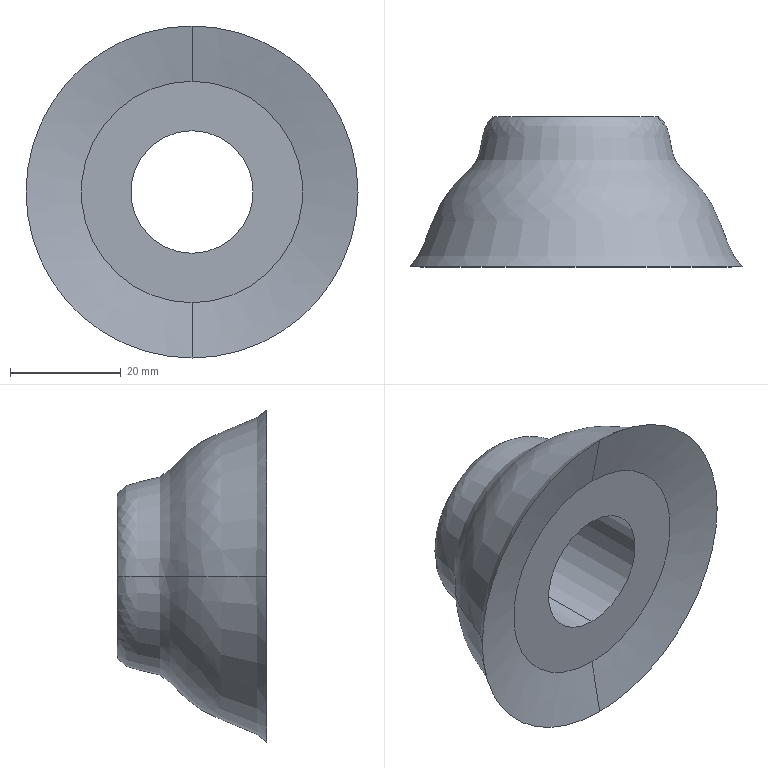Part | STEP file | ASND-0110-6.1aq | 1 solid | 8 faces | box 60 x 27.1 x 60 mm | volume 30806 mm3 | spline 2 | cylinder 2 | cone 2 | plane 2 | commonest cylinder face diameters 22.172 x2
STEP:
#1=CARTESIAN_POINT('',(0.,0.,0.));
#2=DIRECTION('',(0.,0.,1.));
#3=DIRECTION('',(1.,0.,0.));
#4=AXIS2_PLACEMENT_3D('',#1,#2,#3);
#5=CARTESIAN_POINT('',(-30.,-2.,0.));
#6=VERTEX_POINT('',#5);
#7=CARTESIAN_POINT('',(0.,-2.,-30.));
#8=VERTEX_POINT('',#7);
#9=CARTESIAN_POINT('',(0.,-2.,0.));
#10=DIRECTION('',(0.,-1.,0.));
#11=DIRECTION('',(0.,0.,-1.));
#12=AXIS2_PLACEMENT_3D('',#9,#10,#11);
#13=CIRCLE('',#12,30.);
#14=CARTESIAN_POINT('',(30.,-2.,0.));
#15=CARTESIAN_POINT('',(30.,-2.,30.));
#16=CARTESIAN_POINT('',(0.,-2.,30.));
#17=CARTESIAN_POINT('',(-30.,-2.,30.));
#18=CARTESIAN_POINT('',(-30.,-2.,0.));
#19=CARTESIAN_POINT('',(-30.,-2.,-30.));
#20=CARTESIAN_POINT('',(0.,-2.,-30.));
#21=CARTESIAN_POINT('',(30.,-2.,-30.));
#22=CARTESIAN_POINT('',(30.,-2.,0.));
#23=CARTESIAN_POINT('',(27.787,0.3256,0.));
#24=CARTESIAN_POINT('',(27.787,0.3256,27.787));
#25=CARTESIAN_POINT('',(0.,0.3256,27.787));
#26=CARTESIAN_POINT('',(-27.787,0.3256,27.787));
#27=CARTESIAN_POINT('',(-27.787,0.3256,0.));
#28=CARTESIAN_POINT('',(-27.787,0.3256,-27.787));
#29=CARTESIAN_POINT('',(0.,0.3256,-27.787));
#30=CARTESIAN_POINT('',(27.787,0.3256,-27.787));
#31=CARTESIAN_POINT('',(27.787,0.3256,0.));
#32=CARTESIAN_POINT('',(26.457,6.106,0.));
#33=CARTESIAN_POINT('',(26.457,6.106,26.457));
#34=CARTESIAN_POINT('',(0.,6.106,26.457));
#35=CARTESIAN_POINT('',(-26.457,6.106,26.457));
#36=CARTESIAN_POINT('',(-26.457,6.106,0.));
#37=CARTESIAN_POINT('',(-26.457,6.106,-26.457));
#38=CARTESIAN_POINT('',(0.,6.106,-26.457));
#39=CARTESIAN_POINT('',(26.457,6.106,-26.457));
#40=CARTESIAN_POINT('',(26.457,6.106,0.));
#41=CARTESIAN_POINT('',(22.66,12.882,0.));
#42=CARTESIAN_POINT('',(22.66,12.882,22.66));
#43=CARTESIAN_POINT('',(0.,12.882,22.66));
#44=CARTESIAN_POINT('',(-22.66,12.882,22.66));
#45=CARTESIAN_POINT('',(-22.66,12.882,0.));
#46=CARTESIAN_POINT('',(-22.66,12.882,-22.66));
#47=CARTESIAN_POINT('',(0.,12.882,-22.66));
#48=CARTESIAN_POINT('',(22.66,12.882,-22.66));
#49=CARTESIAN_POINT('',(22.66,12.882,0.));
#50=CARTESIAN_POINT('',(16.242,17.513,0.));
#51=CARTESIAN_POINT('',(16.242,17.513,16.242));
#52=CARTESIAN_POINT('',(0.,17.513,16.242));
#53=CARTESIAN_POINT('',(-16.242,17.513,16.242));
#54=CARTESIAN_POINT('',(-16.242,17.513,0.));
#55=CARTESIAN_POINT('',(-16.242,17.513,-16.242));
#56=CARTESIAN_POINT('',(0.,17.513,-16.242));
#57=CARTESIAN_POINT('',(16.242,17.513,-16.242));
#58=CARTESIAN_POINT('',(16.242,17.513,0.));
#59=CARTESIAN_POINT('',(17.432,23.181,0.));
#60=CARTESIAN_POINT('',(17.432,23.181,17.432));
#61=CARTESIAN_POINT('',(0.,23.181,17.432));
#62=CARTESIAN_POINT('',(-17.432,23.181,17.432));
#63=CARTESIAN_POINT('',(-17.432,23.181,0.));
#64=CARTESIAN_POINT('',(-17.432,23.181,-17.432));
#65=CARTESIAN_POINT('',(0.,23.181,-17.432));
#66=CARTESIAN_POINT('',(17.432,23.181,-17.432));
#67=CARTESIAN_POINT('',(17.432,23.181,0.));
#68=CARTESIAN_POINT('',(15.,25.1,0.));
#69=CARTESIAN_POINT('',(15.,25.1,15.));
#70=CARTESIAN_POINT('',(0.,25.1,15.));
#71=CARTESIAN_POINT('',(-15.,25.1,15.));
#72=CARTESIAN_POINT('',(-15.,25.1,0.));
#73=CARTESIAN_POINT('',(-15.,25.1,-15.));
#74=CARTESIAN_POINT('',(0.,25.1,-15.));
#75=CARTESIAN_POINT('',(15.,25.1,-15.));
#76=CARTESIAN_POINT('',(15.,25.1,0.));
#77=(BOUNDED_SURFACE()B_SPLINE_SURFACE(3,2,((#14,#15,#16,#17,#18,#19,#20,#21,#22),(#23,#24,#25,#26,#27,#28,#29,#30,#31),(#32,#33,#34,#35,#36,#37,#38,#39,#40),(#41,#42,#43,#44,#45,#46,#47,#48,#49),(#50,#51,#52,#53,#54,#55,#56,#57,#58),(#59,#60,#61,#62,#63,#64,#65,#66,#67),(#68,#69,#70,#71,#72,#73,#74,#75,#76)),.UNSPECIFIED.,.F.,.T.,.F.)B_SPLINE_SURFACE_WITH_KNOTS((4,1,1,1,4),(1,2,2,2,2,2,1),(0.,0.2961,0.5565,0.7341,1.),(-1.571,0.,1.571,3.142,4.712,6.283,7.854),.UNSPECIFIED.)GEOMETRIC_REPRESENTATION_ITEM()RATIONAL_B_SPLINE_SURFACE(((1.,0.7071,1.,0.7071,1.,0.7071,1.,0.7071,1.),(1.,0.7071,1.,0.7071,1.,0.7071,1.,0.7071,1.),(1.,0.7071,1.,0.7071,1.,0.7071,1.,0.7071,1.),(1.,0.7071,1.,0.7071,1.,0.7071,1.,0.7071,1.),(1.,0.7071,1.,0.7071,1.,0.7071,1.,0.7071,1.),(1.,0.7071,1.,0.7071,1.,0.7071,1.,0.7071,1.),(1.,0.7071,1.,0.7071,1.,0.7071,1.,0.7071,1.)))REPRESENTATION_ITEM('')SURFACE());
#78=CARTESIAN_POINT('',(0.,3.142));
#79=CARTESIAN_POINT('',(0.,3.168));
#80=CARTESIAN_POINT('',(0.,3.22));
#81=CARTESIAN_POINT('',(0.,3.296));
#82=CARTESIAN_POINT('',(0.,3.37));
#83=CARTESIAN_POINT('',(0.,3.443));
#84=CARTESIAN_POINT('',(0.,3.515));
#85=CARTESIAN_POINT('',(0.,3.585));
#86=CARTESIAN_POINT('',(0.,3.654));
#87=CARTESIAN_POINT('',(0.,3.723));
#88=CARTESIAN_POINT('',(0.,3.791));
#89=CARTESIAN_POINT('',(0.,3.859));
#90=CARTESIAN_POINT('',(0.,3.927));
#91=CARTESIAN_POINT('',(0.,3.995));
#92=CARTESIAN_POINT('',(0.,4.063));
#93=CARTESIAN_POINT('',(0.,4.131));
#94=CARTESIAN_POINT('',(0.,4.199));
#95=CARTESIAN_POINT('',(0.,4.269));
#96=CARTESIAN_POINT('',(0.,4.339));
#97=CARTESIAN_POINT('',(0.,4.411));
#98=CARTESIAN_POINT('',(0.,4.483));
#99=CARTESIAN_POINT('',(0.,4.558));
#100=CARTESIAN_POINT('',(0.,4.634));
#101=CARTESIAN_POINT('',(0.,4.686));
#102=CARTESIAN_POINT('',(0.,4.712));
#103=B_SPLINE_CURVE_WITH_KNOTS('',3,(#78,#79,#80,#81,#82,#83,#84,#85,#86,#87,#88,#89,#90,#91,#92,#93,#94,#95,#96,#97,#98,#99,#100,#101,#102),.UNSPECIFIED.,.F.,.F.,(4,1,1,1,1,1,1,1,1,1,1,1,1,1,1,1,1,1,1,1,1,1,4),(4.712,4.784,4.855,4.927,4.998,5.069,5.141,5.212,5.284,5.355,5.426,5.498,5.569,5.641,5.712,5.783,5.855,5.926,5.998,6.069,6.14,6.212,6.283),.QUASI_UNIFORM_KNOTS.);
#104=(GEOMETRIC_REPRESENTATION_CONTEXT(2)PARAMETRIC_REPRESENTATION_CONTEXT()REPRESENTATION_CONTEXT('',''));
#105=DEFINITIONAL_REPRESENTATION('',(#103),#104);
#106=PCURVE('',#77,#105);
#107=CARTESIAN_POINT('',(0.,0.,0.));
#108=DIRECTION('',(0.,-1.,0.));
#109=DIRECTION('',(0.,0.,-1.));
#110=AXIS2_PLACEMENT_3D('',#107,#108,#109);
#111=CONICAL_SURFACE('',#110,20.,1.373);
#112=CARTESIAN_POINT('',(0.,2.));
#113=DIRECTION('',(1.,0.));
#114=VECTOR('',#113,1.);
#115=LINE('',#112,#114);
#116=(GEOMETRIC_REPRESENTATION_CONTEXT(2)PARAMETRIC_REPRESENTATION_CONTEXT()REPRESENTATION_CONTEXT('',''));
#117=DEFINITIONAL_REPRESENTATION('',(#115),#116);
#118=PCURVE('',#111,#117);
#119=SURFACE_CURVE('',#13,(#106,#118),.PCURVE_S1.);
#120=EDGE_CURVE('',#6,#8,#119,.T.);
#121=ORIENTED_EDGE('',*,*,#120,.F.);
#122=CARTESIAN_POINT('',(-15.,25.1,0.));
#123=VERTEX_POINT('',#122);
#124=CARTESIAN_POINT('',(-30.,-2.,0.));
#125=CARTESIAN_POINT('',(-27.787,0.3256,0.));
#126=CARTESIAN_POINT('',(-26.457,6.106,0.));
#127=CARTESIAN_POINT('',(-22.66,12.882,0.));
#128=CARTESIAN_POINT('',(-16.242,17.513,0.));
#129=CARTESIAN_POINT('',(-17.432,23.181,0.));
#130=CARTESIAN_POINT('',(-15.,25.1,0.));
#131=B_SPLINE_CURVE_WITH_KNOTS('',3,(#124,#125,#126,#127,#128,#129,#130),.UNSPECIFIED.,.F.,.F.,(4,1,1,1,4),(0.,0.2961,0.5565,0.7341,1.),.UNSPECIFIED.);
#132=CARTESIAN_POINT('',(0.,3.142));
#133=DIRECTION('',(1.,0.));
#134=VECTOR('',#133,1.);
#135=LINE('',#132,#134);
#136=(GEOMETRIC_REPRESENTATION_CONTEXT(2)PARAMETRIC_REPRESENTATION_CONTEXT()REPRESENTATION_CONTEXT('',''));
#137=DEFINITIONAL_REPRESENTATION('',(#135),#136);
#138=PCURVE('',#77,#137);
#139=CARTESIAN_POINT('',(30.,-2.,0.));
#140=CARTESIAN_POINT('',(30.,-2.,30.));
#141=CARTESIAN_POINT('',(0.,-2.,30.));
#142=CARTESIAN_POINT('',(-30.,-2.,30.));
#143=CARTESIAN_POINT('',(-30.,-2.,0.));
#144=CARTESIAN_POINT('',(-30.,-2.,-30.));
#145=CARTESIAN_POINT('',(0.,-2.,-30.));
#146=CARTESIAN_POINT('',(30.,-2.,-30.));
#147=CARTESIAN_POINT('',(30.,-2.,0.));
#148=CARTESIAN_POINT('',(27.787,0.3256,0.));
#149=CARTESIAN_POINT('',(27.787,0.3256,27.787));
#150=CARTESIAN_POINT('',(0.,0.3256,27.787));
#151=CARTESIAN_POINT('',(-27.787,0.3256,27.787));
#152=CARTESIAN_POINT('',(-27.787,0.3256,0.));
#153=CARTESIAN_POINT('',(-27.787,0.3256,-27.787));
#154=CARTESIAN_POINT('',(0.,0.3256,-27.787));
#155=CARTESIAN_POINT('',(27.787,0.3256,-27.787));
#156=CARTESIAN_POINT('',(27.787,0.3256,0.));
#157=CARTESIAN_POINT('',(26.457,6.106,0.));
#158=CARTESIAN_POINT('',(26.457,6.106,26.457));
#159=CARTESIAN_POINT('',(0.,6.106,26.457));
#160=CARTESIAN_POINT('',(-26.457,6.106,26.457));
#161=CARTESIAN_POINT('',(-26.457,6.106,0.));
#162=CARTESIAN_POINT('',(-26.457,6.106,-26.457));
#163=CARTESIAN_POINT('',(0.,6.106,-26.457));
#164=CARTESIAN_POINT('',(26.457,6.106,-26.457));
#165=CARTESIAN_POINT('',(26.457,6.106,0.));
#166=CARTESIAN_POINT('',(22.66,12.882,0.));
#167=CARTESIAN_POINT('',(22.66,12.882,22.66));
#168=CARTESIAN_POINT('',(0.,12.882,22.66));
#169=CARTESIAN_POINT('',(-22.66,12.882,22.66));
#170=CARTESIAN_POINT('',(-22.66,12.882,0.));
#171=CARTESIAN_POINT('',(-22.66,12.882,-22.66));
#172=CARTESIAN_POINT('',(0.,12.882,-22.66));
#173=CARTESIAN_POINT('',(22.66,12.882,-22.66));
#174=CARTESIAN_POINT('',(22.66,12.882,0.));
#175=CARTESIAN_POINT('',(16.242,17.513,0.));
#176=CARTESIAN_POINT('',(16.242,17.513,16.242));
#177=CARTESIAN_POINT('',(0.,17.513,16.242));
#178=CARTESIAN_POINT('',(-16.242,17.513,16.242));
#179=CARTESIAN_POINT('',(-16.242,17.513,0.));
#180=CARTESIAN_POINT('',(-16.242,17.513,-16.242));
#181=CARTESIAN_POINT('',(0.,17.513,-16.242));
#182=CARTESIAN_POINT('',(16.242,17.513,-16.242));
#183=CARTESIAN_POINT('',(16.242,17.513,0.));
#184=CARTESIAN_POINT('',(17.432,23.181,0.));
#185=CARTESIAN_POINT('',(17.432,23.181,17.432));
#186=CARTESIAN_POINT('',(0.,23.181,17.432));
#187=CARTESIAN_POINT('',(-17.432,23.181,17.432));
#188=CARTESIAN_POINT('',(-17.432,23.181,0.));
#189=CARTESIAN_POINT('',(-17.432,23.181,-17.432));
#190=CARTESIAN_POINT('',(0.,23.181,-17.432));
#191=CARTESIAN_POINT('',(17.432,23.181,-17.432));
#192=CARTESIAN_POINT('',(17.432,23.181,0.));
#193=CARTESIAN_POINT('',(15.,25.1,0.));
#194=CARTESIAN_POINT('',(15.,25.1,15.));
#195=CARTESIAN_POINT('',(0.,25.1,15.));
#196=CARTESIAN_POINT('',(-15.,25.1,15.));
#197=CARTESIAN_POINT('',(-15.,25.1,0.));
#198=CARTESIAN_POINT('',(-15.,25.1,-15.));
#199=CARTESIAN_POINT('',(0.,25.1,-15.));
#200=CARTESIAN_POINT('',(15.,25.1,-15.));
#201=CARTESIAN_POINT('',(15.,25.1,0.));
#202=(BOUNDED_SURFACE()B_SPLINE_SURFACE(3,2,((#139,#140,#141,#142,#143,#144,#145,#146,#147),(#148,#149,#150,#151,#152,#153,#154,#155,#156),(#157,#158,#159,#160,#161,#162,#163,#164,#165),(#166,#167,#168,#169,#170,#171,#172,#173,#174),(#175,#176,#177,#178,#179,#180,#181,#182,#183),(#184,#185,#186,#187,#188,#189,#190,#191,#192),(#193,#194,#195,#196,#197,#198,#199,#200,#201)),.UNSPECIFIED.,.F.,.T.,.F.)B_SPLINE_SURFACE_WITH_KNOTS((4,1,1,1,4),(1,2,2,2,2,2,1),(0.,0.2961,0.5565,0.7341,1.),(-1.571,0.,1.571,3.142,4.712,6.283,7.854),.UNSPECIFIED.)GEOMETRIC_REPRESENTATION_ITEM()RATIONAL_B_SPLINE_SURFACE(((1.,0.7071,1.,0.7071,1.,0.7071,1.,0.7071,1.),(1.,0.7071,1.,0.7071,1.,0.7071,1.,0.7071,1.),(1.,0.7071,1.,0.7071,1.,0.7071,1.,0.7071,1.),(1.,0.7071,1.,0.7071,1.,0.7071,1.,0.7071,1.),(1.,0.7071,1.,0.7071,1.,0.7071,1.,0.7071,1.),(1.,0.7071,1.,0.7071,1.,0.7071,1.,0.7071,1.),(1.,0.7071,1.,0.7071,1.,0.7071,1.,0.7071,1.)))REPRESENTATION_ITEM('')SURFACE());
#203=CARTESIAN_POINT('',(0.,3.142));
#204=DIRECTION('',(1.,0.));
#205=VECTOR('',#204,1.);
#206=LINE('',#203,#205);
#207=(GEOMETRIC_REPRESENTATION_CONTEXT(2)PARAMETRIC_REPRESENTATION_CONTEXT()REPRESENTATION_CONTEXT('',''));
#208=DEFINITIONAL_REPRESENTATION('',(#206),#207);
#209=PCURVE('',#202,#208);
#210=SURFACE_CURVE('',#131,(#138,#209),.PCURVE_S1.);
#211=EDGE_CURVE('',#6,#123,#210,.T.);
#212=ORIENTED_EDGE('',*,*,#211,.T.);
#213=CARTESIAN_POINT('',(15.,25.1,0.));
#214=VERTEX_POINT('',#213);
#215=CARTESIAN_POINT('',(0.,25.1,0.));
#216=DIRECTION('',(0.,-1.,0.));
#217=DIRECTION('',(0.,0.,-1.));
#218=AXIS2_PLACEMENT_3D('',#215,#216,#217);
#219=CIRCLE('',#218,15.);
#220=CARTESIAN_POINT('',(1.,3.142));
#221=CARTESIAN_POINT('',(1.,3.194));
#222=CARTESIAN_POINT('',(1.,3.297));
#223=CARTESIAN_POINT('',(1.,3.444));
#224=CARTESIAN_POINT('',(1.,3.585));
#225=CARTESIAN_POINT('',(1.,3.723));
#226=CARTESIAN_POINT('',(1.,3.859));
#227=CARTESIAN_POINT('',(1.,3.995));
#228=CARTESIAN_POINT('',(1.,4.131));
#229=CARTESIAN_POINT('',(1.,4.268));
#230=CARTESIAN_POINT('',(1.,4.41));
#231=CARTESIAN_POINT('',(1.,4.556));
#232=CARTESIAN_POINT('',(1.,4.712));
#233=CARTESIAN_POINT('',(1.,4.868));
#234=CARTESIAN_POINT('',(1.,5.015));
#235=CARTESIAN_POINT('',(1.,5.156));
#236=CARTESIAN_POINT('',(1.,5.294));
#237=CARTESIAN_POINT('',(1.,5.43));
#238=CARTESIAN_POINT('',(1.,5.565));
#239=CARTESIAN_POINT('',(1.,5.701));
#240=CARTESIAN_POINT('',(1.,5.839));
#241=CARTESIAN_POINT('',(1.,5.981));
#242=CARTESIAN_POINT('',(1.,6.128));
#243=CARTESIAN_POINT('',(1.,6.23));
#244=CARTESIAN_POINT('',(1.,6.283));
#245=B_SPLINE_CURVE_WITH_KNOTS('',3,(#220,#221,#222,#223,#224,#225,#226,#227,#228,#229,#230,#231,#232,#233,#234,#235,#236,#237,#238,#239,#240,#241,#242,#243,#244),.UNSPECIFIED.,.F.,.F.,(4,1,1,1,1,1,1,1,1,1,1,1,1,1,1,1,1,1,1,1,1,1,4),(4.712,4.855,4.998,5.141,5.284,5.426,5.569,5.712,5.855,5.998,6.14,6.283,6.426,6.569,6.712,6.854,6.997,7.14,7.283,7.426,7.568,7.711,7.854),.QUASI_UNIFORM_KNOTS.);
#246=(GEOMETRIC_REPRESENTATION_CONTEXT(2)PARAMETRIC_REPRESENTATION_CONTEXT()REPRESENTATION_CONTEXT('',''));
#247=DEFINITIONAL_REPRESENTATION('',(#245),#246);
#248=PCURVE('',#77,#247);
#249=CARTESIAN_POINT('',(0.,25.1,0.));
#250=DIRECTION('',(0.,1.,0.));
#251=DIRECTION('',(0.7071,0.,0.7071));
#252=AXIS2_PLACEMENT_3D('',#249,#250,#251);
#253=PLANE('',#252);
#254=CARTESIAN_POINT('',(-10.607,10.607));
#255=CARTESIAN_POINT('',(7.765,28.978));
#256=CARTESIAN_POINT('',(14.489,3.882));
#257=CARTESIAN_POINT('',(21.213,-21.213));
#258=CARTESIAN_POINT('',(-3.882,-14.489));
#259=CARTESIAN_POINT('',(-28.978,-7.765));
#260=CARTESIAN_POINT('',(-10.607,10.607));
#261=(BOUNDED_CURVE()B_SPLINE_CURVE(2,(#254,#255,#256,#257,#258,#259,#260),.UNSPECIFIED.,.T.,.F.)B_SPLINE_CURVE_WITH_KNOTS((1,2,2,2,2,1),(-2.094,0.,2.094,4.189,6.283,8.378),.UNSPECIFIED.)CURVE()GEOMETRIC_REPRESENTATION_ITEM()RATIONAL_B_SPLINE_CURVE((1.,0.5,1.,0.5,1.,0.5,1.))REPRESENTATION_ITEM(''));
#262=(GEOMETRIC_REPRESENTATION_CONTEXT(2)PARAMETRIC_REPRESENTATION_CONTEXT()REPRESENTATION_CONTEXT('',''));
#263=DEFINITIONAL_REPRESENTATION('',(#261),#262);
#264=PCURVE('',#253,#263);
#265=SURFACE_CURVE('',#219,(#248,#264),.PCURVE_S1.);
#266=EDGE_CURVE('',#123,#214,#265,.T.);
#267=ORIENTED_EDGE('',*,*,#266,.T.);
#268=CARTESIAN_POINT('',(30.,-2.,0.));
#269=VERTEX_POINT('',#268);
#270=CARTESIAN_POINT('',(30.,-2.,0.));
#271=CARTESIAN_POINT('',(27.787,0.3256,0.));
#272=CARTESIAN_POINT('',(26.457,6.106,0.));
#273=CARTESIAN_POINT('',(22.66,12.882,0.));
#274=CARTESIAN_POINT('',(16.242,17.513,0.));
#275=CARTESIAN_POINT('',(17.432,23.181,0.));
#276=CARTESIAN_POINT('',(15.,25.1,0.));
#277=B_SPLINE_CURVE_WITH_KNOTS('',3,(#270,#271,#272,#273,#274,#275,#276),.UNSPECIFIED.,.F.,.F.,(4,1,1,1,4),(0.,0.2961,0.5565,0.7341,1.),.UNSPECIFIED.);
#278=CARTESIAN_POINT('',(0.,6.283));
#279=DIRECTION('',(1.,0.));
#280=VECTOR('',#279,1.);
#281=LINE('',#278,#280);
#282=(GEOMETRIC_REPRESENTATION_CONTEXT(2)PARAMETRIC_REPRESENTATION_CONTEXT()REPRESENTATION_CONTEXT('',''));
#283=DEFINITIONAL_REPRESENTATION('',(#281),#282);
#284=PCURVE('',#77,#283);
#285=CARTESIAN_POINT('',(0.,0.));
#286=DIRECTION('',(1.,0.));
#287=VECTOR('',#286,1.);
#288=LINE('',#285,#287);
#289=(GEOMETRIC_REPRESENTATION_CONTEXT(2)PARAMETRIC_REPRESENTATION_CONTEXT()REPRESENTATION_CONTEXT('',''));
#290=DEFINITIONAL_REPRESENTATION('',(#288),#289);
#291=PCURVE('',#202,#290);
#292=SURFACE_CURVE('',#277,(#284,#291),.PCURVE_S1.);
#293=EDGE_CURVE('',#269,#214,#292,.T.);
#294=ORIENTED_EDGE('',*,*,#293,.F.);
#295=CARTESIAN_POINT('',(0.,-2.,0.));
#296=DIRECTION('',(0.,-1.,0.));
#297=DIRECTION('',(0.,0.,-1.));
#298=AXIS2_PLACEMENT_3D('',#295,#296,#297);
#299=CIRCLE('',#298,30.);
#300=CARTESIAN_POINT('',(0.,4.712));
#301=CARTESIAN_POINT('',(0.,4.739));
#302=CARTESIAN_POINT('',(0.,4.791));
#303=CARTESIAN_POINT('',(0.,4.867));
#304=CARTESIAN_POINT('',(0.,4.941));
#305=CARTESIAN_POINT('',(0.,5.014));
#306=CARTESIAN_POINT('',(0.,5.085));
#307=CARTESIAN_POINT('',(0.,5.156));
#308=CARTESIAN_POINT('',(0.,5.225));
#309=CARTESIAN_POINT('',(0.,5.294));
#310=CARTESIAN_POINT('',(0.,5.362));
#311=CARTESIAN_POINT('',(0.,5.43));
#312=CARTESIAN_POINT('',(0.,5.498));
#313=CARTESIAN_POINT('',(0.,5.565));
#314=CARTESIAN_POINT('',(0.,5.633));
#315=CARTESIAN_POINT('',(0.,5.702));
#316=CARTESIAN_POINT('',(0.,5.77));
#317=CARTESIAN_POINT('',(0.,5.84));
#318=CARTESIAN_POINT('',(0.,5.91));
#319=CARTESIAN_POINT('',(0.,5.982));
#320=CARTESIAN_POINT('',(0.,6.054));
#321=CARTESIAN_POINT('',(0.,6.129));
#322=CARTESIAN_POINT('',(0.,6.205));
#323=CARTESIAN_POINT('',(0.,6.257));
#324=CARTESIAN_POINT('',(0.,6.283));
#325=B_SPLINE_CURVE_WITH_KNOTS('',3,(#300,#301,#302,#303,#304,#305,#306,#307,#308,#309,#310,#311,#312,#313,#314,#315,#316,#317,#318,#319,#320,#321,#322,#323,#324),.UNSPECIFIED.,.F.,.F.,(4,1,1,1,1,1,1,1,1,1,1,1,1,1,1,1,1,1,1,1,1,1,4),(0.,0.0714,0.1428,0.2142,0.2856,0.357,0.4284,0.4998,0.5712,0.6426,0.714,0.7854,0.8568,0.9282,0.9996,1.071,1.142,1.214,1.285,1.357,1.428,1.499,1.571),.QUASI_UNIFORM_KNOTS.);
#326=(GEOMETRIC_REPRESENTATION_CONTEXT(2)PARAMETRIC_REPRESENTATION_CONTEXT()REPRESENTATION_CONTEXT('',''));
#327=DEFINITIONAL_REPRESENTATION('',(#325),#326);
#328=PCURVE('',#77,#327);
#329=CARTESIAN_POINT('',(0.,0.,0.));
#330=DIRECTION('',(0.,-1.,0.));
#331=DIRECTION('',(0.,0.,-1.));
#332=AXIS2_PLACEMENT_3D('',#329,#330,#331);
#333=CONICAL_SURFACE('',#332,20.,1.373);
#334=CARTESIAN_POINT('',(0.,2.));
#335=DIRECTION('',(1.,0.));
#336=VECTOR('',#335,1.);
#337=LINE('',#334,#336);
#338=(GEOMETRIC_REPRESENTATION_CONTEXT(2)PARAMETRIC_REPRESENTATION_CONTEXT()REPRESENTATION_CONTEXT('',''));
#339=DEFINITIONAL_REPRESENTATION('',(#337),#338);
#340=PCURVE('',#333,#339);
#341=SURFACE_CURVE('',#299,(#328,#340),.PCURVE_S1.);
#342=EDGE_CURVE('',#8,#269,#341,.T.);
#343=ORIENTED_EDGE('',*,*,#342,.F.);
#344=EDGE_LOOP('',(#121,#212,#267,#294,#343));
#345=FACE_BOUND('',#344,.T.);
#346=ADVANCED_FACE('',(#345),#77,.T.);
#347=CARTESIAN_POINT('',(0.,25.1,-11.086));
#348=VERTEX_POINT('',#347);
#349=CARTESIAN_POINT('',(0.,0.,-11.086));
#350=VERTEX_POINT('',#349);
#351=CARTESIAN_POINT('',(0.,40.,-11.086));
#352=DIRECTION('',(0.,-1.,0.));
#353=VECTOR('',#352,1.);
#354=LINE('',#351,#353);
#355=CARTESIAN_POINT('',(0.,40.,0.));
#356=DIRECTION('',(0.,-1.,0.));
#357=DIRECTION('',(0.,0.,-1.));
#358=AXIS2_PLACEMENT_3D('',#355,#356,#357);
#359=CYLINDRICAL_SURFACE('',#358,11.086);
#360=CARTESIAN_POINT('',(6.283,0.));
#361=DIRECTION('',(0.,1.));
#362=VECTOR('',#361,1.);
#363=LINE('',#360,#362);
#364=(GEOMETRIC_REPRESENTATION_CONTEXT(2)PARAMETRIC_REPRESENTATION_CONTEXT()REPRESENTATION_CONTEXT('',''));
#365=DEFINITIONAL_REPRESENTATION('',(#363),#364);
#366=PCURVE('',#359,#365);
#367=CARTESIAN_POINT('',(0.,40.,0.));
#368=DIRECTION('',(0.,-1.,0.));
#369=DIRECTION('',(0.,0.,-1.));
#370=AXIS2_PLACEMENT_3D('',#367,#368,#369);
#371=CYLINDRICAL_SURFACE('',#370,11.086);
#372=CARTESIAN_POINT('',(0.,0.));
#373=DIRECTION('',(0.,1.));
#374=VECTOR('',#373,1.);
#375=LINE('',#372,#374);
#376=(GEOMETRIC_REPRESENTATION_CONTEXT(2)PARAMETRIC_REPRESENTATION_CONTEXT()REPRESENTATION_CONTEXT('',''));
#377=DEFINITIONAL_REPRESENTATION('',(#375),#376);
#378=PCURVE('',#371,#377);
#379=SURFACE_CURVE('',#354,(#366,#378),.PCURVE_S1.);
#380=EDGE_CURVE('',#348,#350,#379,.T.);
#381=ORIENTED_EDGE('',*,*,#380,.T.);
#382=CARTESIAN_POINT('',(0.,0.,11.086));
#383=VERTEX_POINT('',#382);
#384=CARTESIAN_POINT('',(0.,0.,0.));
#385=DIRECTION('',(0.,-1.,0.));
#386=DIRECTION('',(0.,0.,-1.));
#387=AXIS2_PLACEMENT_3D('',#384,#385,#386);
#388=CIRCLE('',#387,11.086);
#389=CARTESIAN_POINT('',(0.,40.));
#390=DIRECTION('',(1.,0.));
#391=VECTOR('',#390,1.);
#392=LINE('',#389,#391);
#393=(GEOMETRIC_REPRESENTATION_CONTEXT(2)PARAMETRIC_REPRESENTATION_CONTEXT()REPRESENTATION_CONTEXT('',''));
#394=DEFINITIONAL_REPRESENTATION('',(#392),#393);
#395=PCURVE('',#359,#394);
#396=CARTESIAN_POINT('',(0.,0.,0.));
#397=DIRECTION('',(0.,-1.,0.));
#398=DIRECTION('',(0.7071,0.,0.7071));
#399=AXIS2_PLACEMENT_3D('',#396,#397,#398);
#400=PLANE('',#399);
#401=CARTESIAN_POINT('',(0.,0.));
#402=DIRECTION('',(-0.7071,-0.7071));
#403=AXIS2_PLACEMENT_2D('',#401,#402);
#404=CIRCLE('',#403,11.086);
#405=(GEOMETRIC_REPRESENTATION_CONTEXT(2)PARAMETRIC_REPRESENTATION_CONTEXT()REPRESENTATION_CONTEXT('',''));
#406=DEFINITIONAL_REPRESENTATION('',(#404),#405);
#407=PCURVE('',#400,#406);
#408=SURFACE_CURVE('',#388,(#395,#407),.PCURVE_S1.);
#409=EDGE_CURVE('',#383,#350,#408,.T.);
#410=ORIENTED_EDGE('',*,*,#409,.F.);
#411=CARTESIAN_POINT('',(0.,25.1,11.086));
#412=VERTEX_POINT('',#411);
#413=CARTESIAN_POINT('',(0.,40.,11.086));
#414=DIRECTION('',(0.,-1.,0.));
#415=VECTOR('',#414,1.);
#416=LINE('',#413,#415);
#417=CARTESIAN_POINT('',(3.142,0.));
#418=DIRECTION('',(0.,1.));
#419=VECTOR('',#418,1.);
#420=LINE('',#417,#419);
#421=(GEOMETRIC_REPRESENTATION_CONTEXT(2)PARAMETRIC_REPRESENTATION_CONTEXT()REPRESENTATION_CONTEXT('',''));
#422=DEFINITIONAL_REPRESENTATION('',(#420),#421);
#423=PCURVE('',#359,#422);
#424=CARTESIAN_POINT('',(3.142,0.));
#425=DIRECTION('',(0.,1.));
#426=VECTOR('',#425,1.);
#427=LINE('',#424,#426);
#428=(GEOMETRIC_REPRESENTATION_CONTEXT(2)PARAMETRIC_REPRESENTATION_CONTEXT()REPRESENTATION_CONTEXT('',''));
#429=DEFINITIONAL_REPRESENTATION('',(#427),#428);
#430=PCURVE('',#371,#429);
#431=SURFACE_CURVE('',#416,(#423,#430),.PCURVE_S1.);
#432=EDGE_CURVE('',#412,#383,#431,.T.);
#433=ORIENTED_EDGE('',*,*,#432,.F.);
#434=CARTESIAN_POINT('',(0.,25.1,0.));
#435=DIRECTION('',(0.,1.,0.));
#436=DIRECTION('',(0.,0.,1.));
#437=AXIS2_PLACEMENT_3D('',#434,#435,#436);
#438=CIRCLE('',#437,11.086);
#439=CARTESIAN_POINT('',(9.425,14.9));
#440=DIRECTION('',(-1.,0.));
#441=VECTOR('',#440,1.);
#442=LINE('',#439,#441);
#443=(GEOMETRIC_REPRESENTATION_CONTEXT(2)PARAMETRIC_REPRESENTATION_CONTEXT()REPRESENTATION_CONTEXT('',''));
#444=DEFINITIONAL_REPRESENTATION('',(#442),#443);
#445=PCURVE('',#359,#444);
#446=CARTESIAN_POINT('',(0.,0.));
#447=DIRECTION('',(0.7071,-0.7071));
#448=AXIS2_PLACEMENT_2D('',#446,#447);
#449=CIRCLE('',#448,11.086);
#450=(GEOMETRIC_REPRESENTATION_CONTEXT(2)PARAMETRIC_REPRESENTATION_CONTEXT()REPRESENTATION_CONTEXT('',''));
#451=DEFINITIONAL_REPRESENTATION('',(#449),#450);
#452=PCURVE('',#253,#451);
#453=SURFACE_CURVE('',#438,(#445,#452),.PCURVE_S1.);
#454=EDGE_CURVE('',#348,#412,#453,.T.);
#455=ORIENTED_EDGE('',*,*,#454,.F.);
#456=EDGE_LOOP('',(#381,#410,#433,#455));
#457=FACE_BOUND('',#456,.F.);
#458=ADVANCED_FACE('',(#457),#359,.F.);
#459=CARTESIAN_POINT('',(0.,0.,-20.));
#460=VERTEX_POINT('',#459);
#461=CARTESIAN_POINT('',(0.,0.,-20.));
#462=DIRECTION('',(0.,-0.1961,-0.9806));
#463=VECTOR('',#462,1.);
#464=LINE('',#461,#463);
#465=CARTESIAN_POINT('',(6.283,0.));
#466=DIRECTION('',(0.,1.));
#467=VECTOR('',#466,1.);
#468=LINE('',#465,#467);
#469=(GEOMETRIC_REPRESENTATION_CONTEXT(2)PARAMETRIC_REPRESENTATION_CONTEXT()REPRESENTATION_CONTEXT('',''));
#470=DEFINITIONAL_REPRESENTATION('',(#468),#469);
#471=PCURVE('',#111,#470);
#472=CARTESIAN_POINT('',(0.,0.));
#473=DIRECTION('',(0.,1.));
#474=VECTOR('',#473,1.);
#475=LINE('',#472,#474);
#476=(GEOMETRIC_REPRESENTATION_CONTEXT(2)PARAMETRIC_REPRESENTATION_CONTEXT()REPRESENTATION_CONTEXT('',''));
#477=DEFINITIONAL_REPRESENTATION('',(#475),#476);
#478=PCURVE('',#333,#477);
#479=SURFACE_CURVE('',#464,(#471,#478),.PCURVE_S1.);
#480=EDGE_CURVE('',#460,#8,#479,.T.);
#481=ORIENTED_EDGE('',*,*,#480,.T.);
#482=ORIENTED_EDGE('',*,*,#120,.F.);
#483=CARTESIAN_POINT('',(0.,-2.,30.));
#484=VERTEX_POINT('',#483);
#485=CARTESIAN_POINT('',(0.,-2.,0.));
#486=DIRECTION('',(0.,-1.,0.));
#487=DIRECTION('',(0.,0.,-1.));
#488=AXIS2_PLACEMENT_3D('',#485,#486,#487);
#489=CIRCLE('',#488,30.);
#490=CARTESIAN_POINT('',(0.,2.));
#491=DIRECTION('',(1.,0.));
#492=VECTOR('',#491,1.);
#493=LINE('',#490,#492);
#494=(GEOMETRIC_REPRESENTATION_CONTEXT(2)PARAMETRIC_REPRESENTATION_CONTEXT()REPRESENTATION_CONTEXT('',''));
#495=DEFINITIONAL_REPRESENTATION('',(#493),#494);
#496=PCURVE('',#111,#495);
#497=CARTESIAN_POINT('',(0.,1.571));
#498=CARTESIAN_POINT('',(0.,1.597));
#499=CARTESIAN_POINT('',(0.,1.649));
#500=CARTESIAN_POINT('',(0.,1.725));
#501=CARTESIAN_POINT('',(0.,1.8));
#502=CARTESIAN_POINT('',(0.,1.872));
#503=CARTESIAN_POINT('',(0.,1.944));
#504=CARTESIAN_POINT('',(0.,2.014));
#505=CARTESIAN_POINT('',(0.,2.084));
#506=CARTESIAN_POINT('',(0.,2.152));
#507=CARTESIAN_POINT('',(0.,2.221));
#508=CARTESIAN_POINT('',(0.,2.289));
#509=CARTESIAN_POINT('',(0.,2.356));
#510=CARTESIAN_POINT('',(0.,2.424));
#511=CARTESIAN_POINT('',(0.,2.492));
#512=CARTESIAN_POINT('',(0.,2.56));
#513=CARTESIAN_POINT('',(0.,2.629));
#514=CARTESIAN_POINT('',(0.,2.698));
#515=CARTESIAN_POINT('',(0.,2.768));
#516=CARTESIAN_POINT('',(0.,2.84));
#517=CARTESIAN_POINT('',(0.,2.913));
#518=CARTESIAN_POINT('',(0.,2.987));
#519=CARTESIAN_POINT('',(0.,3.063));
#520=CARTESIAN_POINT('',(0.,3.115));
#521=CARTESIAN_POINT('',(0.,3.142));
#522=B_SPLINE_CURVE_WITH_KNOTS('',3,(#497,#498,#499,#500,#501,#502,#503,#504,#505,#506,#507,#508,#509,#510,#511,#512,#513,#514,#515,#516,#517,#518,#519,#520,#521),.UNSPECIFIED.,.F.,.F.,(4,1,1,1,1,1,1,1,1,1,1,1,1,1,1,1,1,1,1,1,1,1,4),(3.142,3.213,3.284,3.356,3.427,3.499,3.57,3.641,3.713,3.784,3.856,3.927,3.998,4.07,4.141,4.213,4.284,4.355,4.427,4.498,4.57,4.641,4.712),.QUASI_UNIFORM_KNOTS.);
#523=(GEOMETRIC_REPRESENTATION_CONTEXT(2)PARAMETRIC_REPRESENTATION_CONTEXT()REPRESENTATION_CONTEXT('',''));
#524=DEFINITIONAL_REPRESENTATION('',(#522),#523);
#525=PCURVE('',#202,#524);
#526=SURFACE_CURVE('',#489,(#496,#525),.PCURVE_S1.);
#527=EDGE_CURVE('',#484,#6,#526,.T.);
#528=ORIENTED_EDGE('',*,*,#527,.F.);
#529=CARTESIAN_POINT('',(0.,0.,20.));
#530=VERTEX_POINT('',#529);
#531=CARTESIAN_POINT('',(0.,0.,20.));
#532=DIRECTION('',(0.,-0.1961,0.9806));
#533=VECTOR('',#532,1.);
#534=LINE('',#531,#533);
#535=CARTESIAN_POINT('',(3.142,0.));
#536=DIRECTION('',(0.,1.));
#537=VECTOR('',#536,1.);
#538=LINE('',#535,#537);
#539=(GEOMETRIC_REPRESENTATION_CONTEXT(2)PARAMETRIC_REPRESENTATION_CONTEXT()REPRESENTATION_CONTEXT('',''));
#540=DEFINITIONAL_REPRESENTATION('',(#538),#539);
#541=PCURVE('',#111,#540);
#542=CARTESIAN_POINT('',(3.142,0.));
#543=DIRECTION('',(0.,1.));
#544=VECTOR('',#543,1.);
#545=LINE('',#542,#544);
#546=(GEOMETRIC_REPRESENTATION_CONTEXT(2)PARAMETRIC_REPRESENTATION_CONTEXT()REPRESENTATION_CONTEXT('',''));
#547=DEFINITIONAL_REPRESENTATION('',(#545),#546);
#548=PCURVE('',#333,#547);
#549=SURFACE_CURVE('',#534,(#541,#548),.PCURVE_S1.);
#550=EDGE_CURVE('',#530,#484,#549,.T.);
#551=ORIENTED_EDGE('',*,*,#550,.F.);
#552=CARTESIAN_POINT('',(0.,0.,0.));
#553=DIRECTION('',(0.,-1.,0.));
#554=DIRECTION('',(0.,0.,-1.));
#555=AXIS2_PLACEMENT_3D('',#552,#553,#554);
#556=CIRCLE('',#555,20.);
#557=CARTESIAN_POINT('',(0.,0.));
#558=DIRECTION('',(1.,0.));
#559=VECTOR('',#558,1.);
#560=LINE('',#557,#559);
#561=(GEOMETRIC_REPRESENTATION_CONTEXT(2)PARAMETRIC_REPRESENTATION_CONTEXT()REPRESENTATION_CONTEXT('',''));
#562=DEFINITIONAL_REPRESENTATION('',(#560),#561);
#563=PCURVE('',#111,#562);
#564=CARTESIAN_POINT('',(0.,0.));
#565=DIRECTION('',(-0.7071,-0.7071));
#566=AXIS2_PLACEMENT_2D('',#564,#565);
#567=CIRCLE('',#566,20.);
#568=(GEOMETRIC_REPRESENTATION_CONTEXT(2)PARAMETRIC_REPRESENTATION_CONTEXT()REPRESENTATION_CONTEXT('',''));
#569=DEFINITIONAL_REPRESENTATION('',(#567),#568);
#570=PCURVE('',#400,#569);
#571=SURFACE_CURVE('',#556,(#563,#570),.PCURVE_S1.);
#572=EDGE_CURVE('',#530,#460,#571,.T.);
#573=ORIENTED_EDGE('',*,*,#572,.T.);
#574=EDGE_LOOP('',(#481,#482,#528,#551,#573));
#575=FACE_BOUND('',#574,.F.);
#576=ADVANCED_FACE('',(#575),#111,.F.);
#577=CARTESIAN_POINT('',(0.,0.,0.));
#578=DIRECTION('',(0.,-1.,0.));
#579=DIRECTION('',(0.,0.,-1.));
#580=AXIS2_PLACEMENT_3D('',#577,#578,#579);
#581=CIRCLE('',#580,20.);
#582=CARTESIAN_POINT('',(0.,0.));
#583=DIRECTION('',(-0.7071,-0.7071));
#584=AXIS2_PLACEMENT_2D('',#582,#583);
#585=CIRCLE('',#584,20.);
#586=(GEOMETRIC_REPRESENTATION_CONTEXT(2)PARAMETRIC_REPRESENTATION_CONTEXT()REPRESENTATION_CONTEXT('',''));
#587=DEFINITIONAL_REPRESENTATION('',(#585),#586);
#588=PCURVE('',#400,#587);
#589=CARTESIAN_POINT('',(0.,0.));
#590=DIRECTION('',(1.,0.));
#591=VECTOR('',#590,1.);
#592=LINE('',#589,#591);
#593=(GEOMETRIC_REPRESENTATION_CONTEXT(2)PARAMETRIC_REPRESENTATION_CONTEXT()REPRESENTATION_CONTEXT('',''));
#594=DEFINITIONAL_REPRESENTATION('',(#592),#593);
#595=PCURVE('',#333,#594);
#596=SURFACE_CURVE('',#581,(#588,#595),.PCURVE_S1.);
#597=EDGE_CURVE('',#460,#530,#596,.T.);
#598=ORIENTED_EDGE('',*,*,#597,.T.);
#599=ORIENTED_EDGE('',*,*,#572,.T.);
#600=EDGE_LOOP('',(#598,#599));
#601=FACE_BOUND('',#600,.T.);
#602=CARTESIAN_POINT('',(0.,0.,0.));
#603=DIRECTION('',(0.,-1.,0.));
#604=DIRECTION('',(0.,0.,-1.));
#605=AXIS2_PLACEMENT_3D('',#602,#603,#604);
#606=CIRCLE('',#605,11.086);
#607=CARTESIAN_POINT('',(0.,0.));
#608=DIRECTION('',(-0.7071,-0.7071));
#609=AXIS2_PLACEMENT_2D('',#607,#608);
#610=CIRCLE('',#609,11.086);
#611=(GEOMETRIC_REPRESENTATION_CONTEXT(2)PARAMETRIC_REPRESENTATION_CONTEXT()REPRESENTATION_CONTEXT('',''));
#612=DEFINITIONAL_REPRESENTATION('',(#610),#611);
#613=PCURVE('',#400,#612);
#614=CARTESIAN_POINT('',(0.,40.));
#615=DIRECTION('',(1.,0.));
#616=VECTOR('',#615,1.);
#617=LINE('',#614,#616);
#618=(GEOMETRIC_REPRESENTATION_CONTEXT(2)PARAMETRIC_REPRESENTATION_CONTEXT()REPRESENTATION_CONTEXT('',''));
#619=DEFINITIONAL_REPRESENTATION('',(#617),#618);
#620=PCURVE('',#371,#619);
#621=SURFACE_CURVE('',#606,(#613,#620),.PCURVE_S1.);
#622=EDGE_CURVE('',#350,#383,#621,.T.);
#623=ORIENTED_EDGE('',*,*,#622,.F.);
#624=ORIENTED_EDGE('',*,*,#409,.F.);
#625=EDGE_LOOP('',(#623,#624));
#626=FACE_BOUND('',#625,.T.);
#627=ADVANCED_FACE('',(#601,#626),#400,.T.);
#628=CARTESIAN_POINT('',(0.,-2.,0.));
#629=DIRECTION('',(0.,-1.,0.));
#630=DIRECTION('',(0.,0.,-1.));
#631=AXIS2_PLACEMENT_3D('',#628,#629,#630);
#632=CIRCLE('',#631,30.);
#633=CARTESIAN_POINT('',(0.,2.));
#634=DIRECTION('',(1.,0.));
#635=VECTOR('',#634,1.);
#636=LINE('',#633,#635);
#637=(GEOMETRIC_REPRESENTATION_CONTEXT(2)PARAMETRIC_REPRESENTATION_CONTEXT()REPRESENTATION_CONTEXT('',''));
#638=DEFINITIONAL_REPRESENTATION('',(#636),#637);
#639=PCURVE('',#333,#638);
#640=CARTESIAN_POINT('',(0.,0.));
#641=CARTESIAN_POINT('',(0.,0.02643));
#642=CARTESIAN_POINT('',(0.,0.07853));
#643=CARTESIAN_POINT('',(0.,0.1546));
#644=CARTESIAN_POINT('',(0.,0.2289));
#645=CARTESIAN_POINT('',(0.,0.3017));
#646=CARTESIAN_POINT('',(0.,0.3731));
#647=CARTESIAN_POINT('',(0.,0.4435));
#648=CARTESIAN_POINT('',(0.,0.5129));
#649=CARTESIAN_POINT('',(0.,0.5816));
#650=CARTESIAN_POINT('',(0.,0.6498));
#651=CARTESIAN_POINT('',(0.,0.7177));
#652=CARTESIAN_POINT('',(0.,0.7854));
#653=CARTESIAN_POINT('',(0.,0.8531));
#654=CARTESIAN_POINT('',(0.,0.921));
#655=CARTESIAN_POINT('',(0.,0.9892));
#656=CARTESIAN_POINT('',(0.,1.058));
#657=CARTESIAN_POINT('',(0.,1.127));
#658=CARTESIAN_POINT('',(0.,1.198));
#659=CARTESIAN_POINT('',(0.,1.269));
#660=CARTESIAN_POINT('',(0.,1.342));
#661=CARTESIAN_POINT('',(0.,1.416));
#662=CARTESIAN_POINT('',(0.,1.492));
#663=CARTESIAN_POINT('',(0.,1.544));
#664=CARTESIAN_POINT('',(0.,1.571));
#665=B_SPLINE_CURVE_WITH_KNOTS('',3,(#640,#641,#642,#643,#644,#645,#646,#647,#648,#649,#650,#651,#652,#653,#654,#655,#656,#657,#658,#659,#660,#661,#662,#663,#664),.UNSPECIFIED.,.F.,.F.,(4,1,1,1,1,1,1,1,1,1,1,1,1,1,1,1,1,1,1,1,1,1,4),(1.571,1.642,1.714,1.785,1.856,1.928,1.999,2.071,2.142,2.213,2.285,2.356,2.428,2.499,2.57,2.642,2.713,2.785,2.856,2.927,2.999,3.07,3.142),.QUASI_UNIFORM_KNOTS.);
#666=(GEOMETRIC_REPRESENTATION_CONTEXT(2)PARAMETRIC_REPRESENTATION_CONTEXT()REPRESENTATION_CONTEXT('',''));
#667=DEFINITIONAL_REPRESENTATION('',(#665),#666);
#668=PCURVE('',#202,#667);
#669=SURFACE_CURVE('',#632,(#639,#668),.PCURVE_S1.);
#670=EDGE_CURVE('',#269,#484,#669,.T.);
#671=ORIENTED_EDGE('',*,*,#670,.F.);
#672=ORIENTED_EDGE('',*,*,#342,.F.);
#673=ORIENTED_EDGE('',*,*,#480,.F.);
#674=ORIENTED_EDGE('',*,*,#597,.T.);
#675=ORIENTED_EDGE('',*,*,#550,.T.);
#676=EDGE_LOOP('',(#671,#672,#673,#674,#675));
#677=FACE_BOUND('',#676,.F.);
#678=ADVANCED_FACE('',(#677),#333,.F.);
#679=ORIENTED_EDGE('',*,*,#211,.F.);
#680=ORIENTED_EDGE('',*,*,#527,.F.);
#681=ORIENTED_EDGE('',*,*,#670,.F.);
#682=ORIENTED_EDGE('',*,*,#293,.T.);
#683=CARTESIAN_POINT('',(0.,25.1,0.));
#684=DIRECTION('',(0.,-1.,0.));
#685=DIRECTION('',(0.,0.,-1.));
#686=AXIS2_PLACEMENT_3D('',#683,#684,#685);
#687=CIRCLE('',#686,15.);
#688=CARTESIAN_POINT('',(1.,0.));
#689=CARTESIAN_POINT('',(1.,0.05284));
#690=CARTESIAN_POINT('',(1.,0.1555));
#691=CARTESIAN_POINT('',(1.,0.3023));
#692=CARTESIAN_POINT('',(1.,0.4439));
#693=CARTESIAN_POINT('',(1.,0.5819));
#694=CARTESIAN_POINT('',(1.,0.7178));
#695=CARTESIAN_POINT('',(1.,0.853));
#696=CARTESIAN_POINT('',(1.,0.9889));
#697=CARTESIAN_POINT('',(1.,1.127));
#698=CARTESIAN_POINT('',(1.,1.269));
#699=CARTESIAN_POINT('',(1.,1.415));
#700=CARTESIAN_POINT('',(1.,1.571));
#701=CARTESIAN_POINT('',(1.,1.727));
#702=CARTESIAN_POINT('',(1.,1.873));
#703=CARTESIAN_POINT('',(1.,2.015));
#704=CARTESIAN_POINT('',(1.,2.153));
#705=CARTESIAN_POINT('',(1.,2.289));
#706=CARTESIAN_POINT('',(1.,2.424));
#707=CARTESIAN_POINT('',(1.,2.56));
#708=CARTESIAN_POINT('',(1.,2.698));
#709=CARTESIAN_POINT('',(1.,2.839));
#710=CARTESIAN_POINT('',(1.,2.986));
#711=CARTESIAN_POINT('',(1.,3.089));
#712=CARTESIAN_POINT('',(1.,3.142));
#713=B_SPLINE_CURVE_WITH_KNOTS('',3,(#688,#689,#690,#691,#692,#693,#694,#695,#696,#697,#698,#699,#700,#701,#702,#703,#704,#705,#706,#707,#708,#709,#710,#711,#712),.UNSPECIFIED.,.F.,.F.,(4,1,1,1,1,1,1,1,1,1,1,1,1,1,1,1,1,1,1,1,1,1,4),(1.571,1.714,1.856,1.999,2.142,2.285,2.428,2.57,2.713,2.856,2.999,3.142,3.284,3.427,3.57,3.713,3.856,3.998,4.141,4.284,4.427,4.57,4.712),.QUASI_UNIFORM_KNOTS.);
#714=(GEOMETRIC_REPRESENTATION_CONTEXT(2)PARAMETRIC_REPRESENTATION_CONTEXT()REPRESENTATION_CONTEXT('',''));
#715=DEFINITIONAL_REPRESENTATION('',(#713),#714);
#716=PCURVE('',#202,#715);
#717=CARTESIAN_POINT('',(-10.607,10.607));
#718=CARTESIAN_POINT('',(7.765,28.978));
#719=CARTESIAN_POINT('',(14.489,3.882));
#720=CARTESIAN_POINT('',(21.213,-21.213));
#721=CARTESIAN_POINT('',(-3.882,-14.489));
#722=CARTESIAN_POINT('',(-28.978,-7.765));
#723=CARTESIAN_POINT('',(-10.607,10.607));
#724=(BOUNDED_CURVE()B_SPLINE_CURVE(2,(#717,#718,#719,#720,#721,#722,#723),.UNSPECIFIED.,.T.,.F.)B_SPLINE_CURVE_WITH_KNOTS((1,2,2,2,2,1),(-2.094,0.,2.094,4.189,6.283,8.378),.UNSPECIFIED.)CURVE()GEOMETRIC_REPRESENTATION_ITEM()RATIONAL_B_SPLINE_CURVE((1.,0.5,1.,0.5,1.,0.5,1.))REPRESENTATION_ITEM(''));
#725=(GEOMETRIC_REPRESENTATION_CONTEXT(2)PARAMETRIC_REPRESENTATION_CONTEXT()REPRESENTATION_CONTEXT('',''));
#726=DEFINITIONAL_REPRESENTATION('',(#724),#725);
#727=PCURVE('',#253,#726);
#728=SURFACE_CURVE('',#687,(#716,#727),.PCURVE_S1.);
#729=EDGE_CURVE('',#214,#123,#728,.T.);
#730=ORIENTED_EDGE('',*,*,#729,.T.);
#731=EDGE_LOOP('',(#679,#680,#681,#682,#730));
#732=FACE_BOUND('',#731,.T.);
#733=ADVANCED_FACE('',(#732),#202,.T.);
#734=ORIENTED_EDGE('',*,*,#729,.F.);
#735=ORIENTED_EDGE('',*,*,#266,.F.);
#736=EDGE_LOOP('',(#734,#735));
#737=FACE_BOUND('',#736,.T.);
#738=ORIENTED_EDGE('',*,*,#454,.F.);
#739=CARTESIAN_POINT('',(0.,25.1,0.));
#740=DIRECTION('',(0.,1.,0.));
#741=DIRECTION('',(0.,0.,1.));
#742=AXIS2_PLACEMENT_3D('',#739,#740,#741);
#743=CIRCLE('',#742,11.086);
#744=CARTESIAN_POINT('',(0.,0.));
#745=DIRECTION('',(0.7071,-0.7071));
#746=AXIS2_PLACEMENT_2D('',#744,#745);
#747=CIRCLE('',#746,11.086);
#748=(GEOMETRIC_REPRESENTATION_CONTEXT(2)PARAMETRIC_REPRESENTATION_CONTEXT()REPRESENTATION_CONTEXT('',''));
#749=DEFINITIONAL_REPRESENTATION('',(#747),#748);
#750=PCURVE('',#253,#749);
#751=CARTESIAN_POINT('',(3.142,14.9));
#752=DIRECTION('',(-1.,0.));
#753=VECTOR('',#752,1.);
#754=LINE('',#751,#753);
#755=(GEOMETRIC_REPRESENTATION_CONTEXT(2)PARAMETRIC_REPRESENTATION_CONTEXT()REPRESENTATION_CONTEXT('',''));
#756=DEFINITIONAL_REPRESENTATION('',(#754),#755);
#757=PCURVE('',#371,#756);
#758=SURFACE_CURVE('',#743,(#750,#757),.PCURVE_S1.);
#759=EDGE_CURVE('',#412,#348,#758,.T.);
#760=ORIENTED_EDGE('',*,*,#759,.F.);
#761=EDGE_LOOP('',(#738,#760));
#762=FACE_BOUND('',#761,.T.);
#763=ADVANCED_FACE('',(#737,#762),#253,.T.);
#764=ORIENTED_EDGE('',*,*,#622,.F.);
#765=ORIENTED_EDGE('',*,*,#380,.F.);
#766=ORIENTED_EDGE('',*,*,#759,.F.);
#767=ORIENTED_EDGE('',*,*,#432,.T.);
#768=EDGE_LOOP('',(#764,#765,#766,#767));
#769=FACE_BOUND('',#768,.F.);
#770=ADVANCED_FACE('',(#769),#371,.F.);
#771=CLOSED_SHELL('',(#346,#458,#576,#627,#678,#733,#763,#770));
#772=MANIFOLD_SOLID_BREP('',#771);
#773=(LENGTH_UNIT()NAMED_UNIT(*)SI_UNIT(.MILLI.,.METRE.));
#774=UNCERTAINTY_MEASURE_WITH_UNIT(LENGTH_MEASURE(0.0000001),#773,'','');
#775=(NAMED_UNIT(*)PLANE_ANGLE_UNIT()SI_UNIT($,.RADIAN.));
#776=(NAMED_UNIT(*)SI_UNIT($,.STERADIAN.)SOLID_ANGLE_UNIT());
#777=(GEOMETRIC_REPRESENTATION_CONTEXT(3)GLOBAL_UNCERTAINTY_ASSIGNED_CONTEXT((#774))GLOBAL_UNIT_ASSIGNED_CONTEXT((#773,#775,#776))REPRESENTATION_CONTEXT('',''));
#778=ADVANCED_BREP_SHAPE_REPRESENTATION('',(#4,#772),#777);